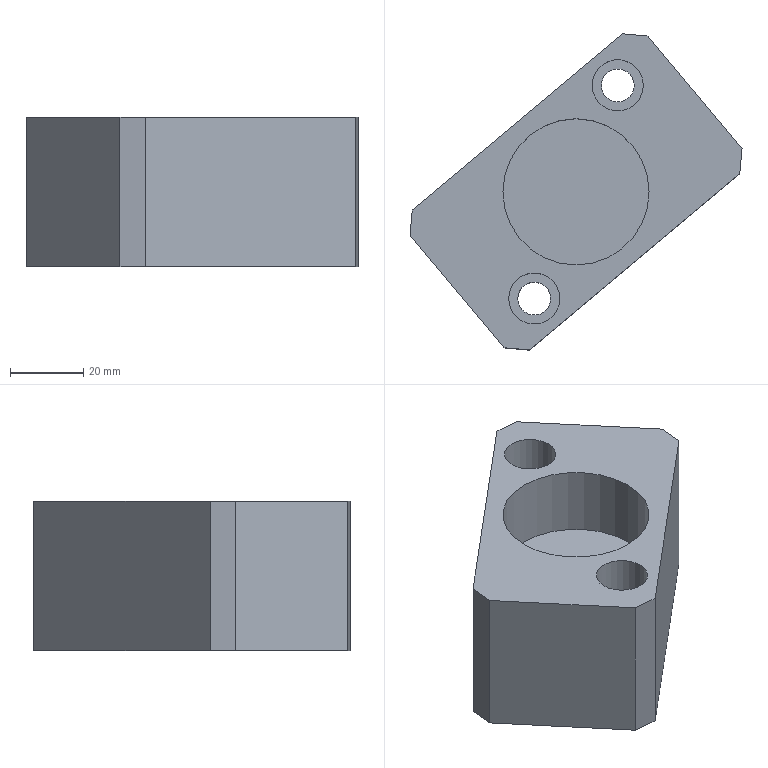Part | NX | features solid 2 | 1 solid | 18 faces | box 90.825 x 86.511 x 41 mm | volume 139314 mm3 | plane 13 | cylinder 5 | commonest cylinder face diameters 9 x2 14 x2 40 x1
STEP:
#1=CARTESIAN_POINT('',(-247.002,-330.511,-169.));
#2=VERTEX_POINT('',#1);
#3=CARTESIAN_POINT('',(-240.002,-330.511,-169.));
#4=DIRECTION('',(0.,0.,-1.));
#5=DIRECTION('',(-1.,0.,0.));
#6=AXIS2_PLACEMENT_3D('',#3,#4,#5);
#7=CIRCLE('',#6,7.);
#8=EDGE_CURVE('',#2,#2,#7,.T.);
#9=ORIENTED_EDGE('',*,*,#8,.T.);
#10=EDGE_LOOP('',(#9));
#11=FACE_BOUND('',#10,.T.);
#12=CARTESIAN_POINT('',(-269.851,-388.846,-169.));
#13=VERTEX_POINT('',#12);
#14=CARTESIAN_POINT('',(-262.851,-388.846,-169.));
#15=DIRECTION('',(0.,0.,-1.));
#16=DIRECTION('',(-1.,0.,0.));
#17=AXIS2_PLACEMENT_3D('',#14,#15,#16);
#18=CIRCLE('',#17,7.);
#19=EDGE_CURVE('',#13,#13,#18,.T.);
#20=ORIENTED_EDGE('',*,*,#19,.T.);
#21=EDGE_LOOP('',(#20));
#22=FACE_BOUND('',#21,.T.);
#23=CARTESIAN_POINT('',(-206.014,-347.681,-169.));
#24=VERTEX_POINT('',#23);
#25=CARTESIAN_POINT('',(-231.725,-317.039,-169.));
#26=VERTEX_POINT('',#25);
#27=CARTESIAN_POINT('',(-206.014,-347.681,-169.));
#28=DIRECTION('',(-0.6428,0.766,0.));
#29=VECTOR('',#28,1000.);
#30=LINE('',#27,#29);
#31=EDGE_CURVE('',#24,#26,#30,.T.);
#32=ORIENTED_EDGE('',*,*,#31,.T.);
#33=CARTESIAN_POINT('',(-238.77,-316.423,-169.));
#34=VERTEX_POINT('',#33);
#35=CARTESIAN_POINT('',(-259.902,-314.574,-169.));
#36=DIRECTION('',(0.9962,-0.08716,0.));
#37=VECTOR('',#36,1000.);
#38=LINE('',#35,#37);
#39=EDGE_CURVE('',#26,#34,#38,.F.);
#40=ORIENTED_EDGE('',*,*,#39,.T.);
#41=CARTESIAN_POINT('',(-296.223,-364.632,-169.));
#42=VERTEX_POINT('',#41);
#43=CARTESIAN_POINT('',(-296.223,-364.632,-169.));
#44=DIRECTION('',(-0.766,-0.6428,0.));
#45=VECTOR('',#44,1000.);
#46=LINE('',#43,#45);
#47=EDGE_CURVE('',#34,#42,#46,.T.);
#48=ORIENTED_EDGE('',*,*,#47,.T.);
#49=CARTESIAN_POINT('',(-296.839,-371.676,-169.));
#50=VERTEX_POINT('',#49);
#51=CARTESIAN_POINT('',(-298.996,-396.331,-169.));
#52=DIRECTION('',(0.08716,0.9962,0.));
#53=VECTOR('',#52,1000.);
#54=LINE('',#51,#53);
#55=EDGE_CURVE('',#42,#50,#54,.F.);
#56=ORIENTED_EDGE('',*,*,#55,.T.);
#57=CARTESIAN_POINT('',(-271.128,-402.318,-169.));
#58=VERTEX_POINT('',#57);
#59=CARTESIAN_POINT('',(-271.128,-402.318,-169.));
#60=DIRECTION('',(0.6428,-0.766,0.));
#61=VECTOR('',#60,1000.);
#62=LINE('',#59,#61);
#63=EDGE_CURVE('',#50,#58,#62,.T.);
#64=ORIENTED_EDGE('',*,*,#63,.T.);
#65=CARTESIAN_POINT('',(-264.084,-402.934,-169.));
#66=VERTEX_POINT('',#65);
#67=CARTESIAN_POINT('',(-267.606,-402.626,-169.));
#68=DIRECTION('',(-0.9962,0.08716,0.));
#69=VECTOR('',#68,1000.);
#70=LINE('',#67,#69);
#71=EDGE_CURVE('',#58,#66,#70,.F.);
#72=ORIENTED_EDGE('',*,*,#71,.T.);
#73=CARTESIAN_POINT('',(-206.63,-354.725,-169.));
#74=VERTEX_POINT('',#73);
#75=CARTESIAN_POINT('',(-264.084,-402.934,-169.));
#76=DIRECTION('',(0.766,0.6428,0.));
#77=VECTOR('',#76,1000.);
#78=LINE('',#75,#77);
#79=EDGE_CURVE('',#66,#74,#78,.T.);
#80=ORIENTED_EDGE('',*,*,#79,.T.);
#81=CARTESIAN_POINT('',(-210.944,-404.034,-169.));
#82=DIRECTION('',(-0.08716,-0.9962,0.));
#83=VECTOR('',#82,1000.);
#84=LINE('',#81,#83);
#85=EDGE_CURVE('',#74,#24,#84,.F.);
#86=ORIENTED_EDGE('',*,*,#85,.T.);
#87=EDGE_LOOP('',(#32,#40,#48,#56,#64,#72,#80,#86));
#88=FACE_BOUND('',#87,.T.);
#89=CARTESIAN_POINT('',(-271.427,-359.679,-169.));
#90=VERTEX_POINT('',#89);
#91=CARTESIAN_POINT('',(-251.427,-359.679,-169.));
#92=DIRECTION('',(0.,0.,1.));
#93=DIRECTION('',(-1.,0.,0.));
#94=AXIS2_PLACEMENT_3D('',#91,#92,#93);
#95=CIRCLE('',#94,20.);
#96=EDGE_CURVE('',#90,#90,#95,.F.);
#97=ORIENTED_EDGE('',*,*,#96,.T.);
#98=EDGE_LOOP('',(#97));
#99=FACE_BOUND('',#98,.T.);
#100=CARTESIAN_POINT('',(-267.297,-399.104,-169.));
#101=DIRECTION('',(0.,0.,1.));
#102=DIRECTION('',(-1.,0.,0.));
#103=AXIS2_PLACEMENT_3D('',#100,#101,#102);
#104=PLANE('',#103);
#105=ADVANCED_FACE('',(#11,#22,#88,#99),#104,.T.);
#106=ORIENTED_EDGE('',*,*,#63,.F.);
#107=CARTESIAN_POINT('',(-296.839,-371.676,-210.));
#108=VERTEX_POINT('',#107);
#109=CARTESIAN_POINT('',(-296.839,-371.676,-209.));
#110=DIRECTION('',(0.,0.,-1.));
#111=VECTOR('',#110,1000.);
#112=LINE('',#109,#111);
#113=EDGE_CURVE('',#50,#108,#112,.T.);
#114=ORIENTED_EDGE('',*,*,#113,.T.);
#115=CARTESIAN_POINT('',(-271.128,-402.318,-210.));
#116=VERTEX_POINT('',#115);
#117=CARTESIAN_POINT('',(-331.881,-329.915,-210.));
#118=DIRECTION('',(0.6428,-0.766,0.));
#119=VECTOR('',#118,1000.);
#120=LINE('',#117,#119);
#121=EDGE_CURVE('',#108,#116,#120,.T.);
#122=ORIENTED_EDGE('',*,*,#121,.T.);
#123=CARTESIAN_POINT('',(-271.128,-402.318,-209.));
#124=DIRECTION('',(0.,0.,1.));
#125=VECTOR('',#124,1000.);
#126=LINE('',#123,#125);
#127=EDGE_CURVE('',#116,#58,#126,.T.);
#128=ORIENTED_EDGE('',*,*,#127,.T.);
#129=EDGE_LOOP('',(#106,#114,#122,#128));
#130=FACE_BOUND('',#129,.T.);
#131=CARTESIAN_POINT('',(-296.839,-371.676,-209.));
#132=DIRECTION('',(-0.766,-0.6428,0.));
#133=DIRECTION('',(0.6428,-0.766,0.));
#134=AXIS2_PLACEMENT_3D('',#131,#132,#133);
#135=PLANE('',#134);
#136=ADVANCED_FACE('',(#130),#135,.T.);
#137=CARTESIAN_POINT('',(-264.084,-402.934,-210.));
#138=VERTEX_POINT('',#137);
#139=CARTESIAN_POINT('',(-206.63,-354.725,-210.));
#140=VERTEX_POINT('',#139);
#141=CARTESIAN_POINT('',(-362.898,-485.85,-210.));
#142=DIRECTION('',(0.766,0.6428,0.));
#143=VECTOR('',#142,1000.);
#144=LINE('',#141,#143);
#145=EDGE_CURVE('',#138,#140,#144,.T.);
#146=ORIENTED_EDGE('',*,*,#145,.T.);
#147=CARTESIAN_POINT('',(-206.63,-354.725,-209.));
#148=DIRECTION('',(0.,0.,1.));
#149=VECTOR('',#148,1000.);
#150=LINE('',#147,#149);
#151=EDGE_CURVE('',#140,#74,#150,.T.);
#152=ORIENTED_EDGE('',*,*,#151,.T.);
#153=ORIENTED_EDGE('',*,*,#79,.F.);
#154=CARTESIAN_POINT('',(-264.084,-402.934,-209.));
#155=DIRECTION('',(0.,0.,-1.));
#156=VECTOR('',#155,1000.);
#157=LINE('',#154,#156);
#158=EDGE_CURVE('',#66,#138,#157,.T.);
#159=ORIENTED_EDGE('',*,*,#158,.T.);
#160=EDGE_LOOP('',(#146,#152,#153,#159));
#161=FACE_BOUND('',#160,.T.);
#162=CARTESIAN_POINT('',(-264.084,-402.934,-209.));
#163=DIRECTION('',(0.6428,-0.766,0.));
#164=DIRECTION('',(0.766,0.6428,0.));
#165=AXIS2_PLACEMENT_3D('',#162,#163,#164);
#166=PLANE('',#165);
#167=ADVANCED_FACE('',(#161),#166,.T.);
#168=CARTESIAN_POINT('',(-206.014,-347.681,-210.));
#169=VERTEX_POINT('',#168);
#170=CARTESIAN_POINT('',(-231.725,-317.039,-210.));
#171=VERTEX_POINT('',#170);
#172=CARTESIAN_POINT('',(-266.767,-275.278,-210.));
#173=DIRECTION('',(-0.6428,0.766,0.));
#174=VECTOR('',#173,1000.);
#175=LINE('',#172,#174);
#176=EDGE_CURVE('',#169,#171,#175,.T.);
#177=ORIENTED_EDGE('',*,*,#176,.T.);
#178=CARTESIAN_POINT('',(-231.725,-317.039,-209.));
#179=DIRECTION('',(0.,0.,1.));
#180=VECTOR('',#179,1000.);
#181=LINE('',#178,#180);
#182=EDGE_CURVE('',#171,#26,#181,.T.);
#183=ORIENTED_EDGE('',*,*,#182,.T.);
#184=ORIENTED_EDGE('',*,*,#31,.F.);
#185=CARTESIAN_POINT('',(-206.014,-347.681,-209.));
#186=DIRECTION('',(0.,0.,-1.));
#187=VECTOR('',#186,1000.);
#188=LINE('',#185,#187);
#189=EDGE_CURVE('',#24,#169,#188,.T.);
#190=ORIENTED_EDGE('',*,*,#189,.T.);
#191=EDGE_LOOP('',(#177,#183,#184,#190));
#192=FACE_BOUND('',#191,.T.);
#193=CARTESIAN_POINT('',(-206.014,-347.681,-209.));
#194=DIRECTION('',(0.766,0.6428,0.));
#195=DIRECTION('',(-0.6428,0.766,0.));
#196=AXIS2_PLACEMENT_3D('',#193,#194,#195);
#197=PLANE('',#196);
#198=ADVANCED_FACE('',(#192),#197,.T.);
#199=ORIENTED_EDGE('',*,*,#47,.F.);
#200=CARTESIAN_POINT('',(-238.77,-316.423,-210.));
#201=VERTEX_POINT('',#200);
#202=CARTESIAN_POINT('',(-238.77,-316.423,-209.));
#203=DIRECTION('',(0.,0.,-1.));
#204=VECTOR('',#203,1000.);
#205=LINE('',#202,#204);
#206=EDGE_CURVE('',#34,#201,#205,.T.);
#207=ORIENTED_EDGE('',*,*,#206,.T.);
#208=CARTESIAN_POINT('',(-296.223,-364.632,-210.));
#209=VERTEX_POINT('',#208);
#210=CARTESIAN_POINT('',(-395.038,-447.548,-210.));
#211=DIRECTION('',(-0.766,-0.6428,0.));
#212=VECTOR('',#211,1000.);
#213=LINE('',#210,#212);
#214=EDGE_CURVE('',#201,#209,#213,.T.);
#215=ORIENTED_EDGE('',*,*,#214,.T.);
#216=CARTESIAN_POINT('',(-296.223,-364.632,-209.));
#217=DIRECTION('',(0.,0.,1.));
#218=VECTOR('',#217,1000.);
#219=LINE('',#216,#218);
#220=EDGE_CURVE('',#209,#42,#219,.T.);
#221=ORIENTED_EDGE('',*,*,#220,.T.);
#222=EDGE_LOOP('',(#199,#207,#215,#221));
#223=FACE_BOUND('',#222,.T.);
#224=CARTESIAN_POINT('',(-238.77,-316.423,-209.));
#225=DIRECTION('',(-0.6428,0.766,0.));
#226=DIRECTION('',(-0.766,-0.6428,0.));
#227=AXIS2_PLACEMENT_3D('',#224,#225,#226);
#228=PLANE('',#227);
#229=ADVANCED_FACE('',(#223),#228,.T.);
#230=CARTESIAN_POINT('',(-244.502,-330.511,-210.));
#231=VERTEX_POINT('',#230);
#232=CARTESIAN_POINT('',(-240.002,-330.511,-210.));
#233=DIRECTION('',(0.,0.,-1.));
#234=DIRECTION('',(-1.,0.,0.));
#235=AXIS2_PLACEMENT_3D('',#232,#233,#234);
#236=CIRCLE('',#235,4.5);
#237=EDGE_CURVE('',#231,#231,#236,.T.);
#238=ORIENTED_EDGE('',*,*,#237,.F.);
#239=EDGE_LOOP('',(#238));
#240=FACE_BOUND('',#239,.T.);
#241=CARTESIAN_POINT('',(-267.351,-388.846,-210.));
#242=VERTEX_POINT('',#241);
#243=CARTESIAN_POINT('',(-262.851,-388.846,-210.));
#244=DIRECTION('',(0.,0.,-1.));
#245=DIRECTION('',(-1.,0.,0.));
#246=AXIS2_PLACEMENT_3D('',#243,#244,#245);
#247=CIRCLE('',#246,4.5);
#248=EDGE_CURVE('',#242,#242,#247,.T.);
#249=ORIENTED_EDGE('',*,*,#248,.F.);
#250=EDGE_LOOP('',(#249));
#251=FACE_BOUND('',#250,.T.);
#252=ORIENTED_EDGE('',*,*,#214,.F.);
#253=CARTESIAN_POINT('',(-231.725,-317.039,-210.));
#254=DIRECTION('',(-0.9962,0.08716,0.));
#255=VECTOR('',#254,1000.);
#256=LINE('',#253,#255);
#257=EDGE_CURVE('',#201,#171,#256,.F.);
#258=ORIENTED_EDGE('',*,*,#257,.T.);
#259=ORIENTED_EDGE('',*,*,#176,.F.);
#260=CARTESIAN_POINT('',(-206.63,-354.725,-210.));
#261=DIRECTION('',(0.08716,0.9962,0.));
#262=VECTOR('',#261,1000.);
#263=LINE('',#260,#262);
#264=EDGE_CURVE('',#169,#140,#263,.F.);
#265=ORIENTED_EDGE('',*,*,#264,.T.);
#266=ORIENTED_EDGE('',*,*,#145,.F.);
#267=CARTESIAN_POINT('',(-271.128,-402.318,-210.));
#268=DIRECTION('',(0.9962,-0.08716,0.));
#269=VECTOR('',#268,1000.);
#270=LINE('',#267,#269);
#271=EDGE_CURVE('',#138,#116,#270,.F.);
#272=ORIENTED_EDGE('',*,*,#271,.T.);
#273=ORIENTED_EDGE('',*,*,#121,.F.);
#274=CARTESIAN_POINT('',(-296.223,-364.632,-210.));
#275=DIRECTION('',(-0.08716,-0.9962,0.));
#276=VECTOR('',#275,1000.);
#277=LINE('',#274,#276);
#278=EDGE_CURVE('',#108,#209,#277,.F.);
#279=ORIENTED_EDGE('',*,*,#278,.T.);
#280=EDGE_LOOP('',(#252,#258,#259,#265,#266,#272,#273,#279));
#281=FACE_BOUND('',#280,.T.);
#282=CARTESIAN_POINT('',(-426.866,-409.617,-210.));
#283=DIRECTION('',(0.,0.,1.));
#284=DIRECTION('',(-1.,0.,0.));
#285=AXIS2_PLACEMENT_3D('',#282,#283,#284);
#286=PLANE('',#285);
#287=ADVANCED_FACE('',(#240,#251,#281),#286,.F.);
#288=ORIENTED_EDGE('',*,*,#271,.F.);
#289=ORIENTED_EDGE('',*,*,#158,.F.);
#290=ORIENTED_EDGE('',*,*,#71,.F.);
#291=ORIENTED_EDGE('',*,*,#127,.F.);
#292=EDGE_LOOP('',(#288,#289,#290,#291));
#293=FACE_BOUND('',#292,.T.);
#294=CARTESIAN_POINT('',(-271.128,-402.318,-209.));
#295=DIRECTION('',(0.08716,0.9962,0.));
#296=DIRECTION('',(-0.9962,0.08716,0.));
#297=AXIS2_PLACEMENT_3D('',#294,#295,#296);
#298=PLANE('',#297);
#299=ADVANCED_FACE('',(#293),#298,.F.);
#300=ORIENTED_EDGE('',*,*,#278,.F.);
#301=ORIENTED_EDGE('',*,*,#113,.F.);
#302=ORIENTED_EDGE('',*,*,#55,.F.);
#303=ORIENTED_EDGE('',*,*,#220,.F.);
#304=EDGE_LOOP('',(#300,#301,#302,#303));
#305=FACE_BOUND('',#304,.T.);
#306=CARTESIAN_POINT('',(-296.223,-364.632,-209.));
#307=DIRECTION('',(0.9962,-0.08716,0.));
#308=DIRECTION('',(0.08716,0.9962,0.));
#309=AXIS2_PLACEMENT_3D('',#306,#307,#308);
#310=PLANE('',#309);
#311=ADVANCED_FACE('',(#305),#310,.F.);
#312=ORIENTED_EDGE('',*,*,#264,.F.);
#313=ORIENTED_EDGE('',*,*,#189,.F.);
#314=ORIENTED_EDGE('',*,*,#85,.F.);
#315=ORIENTED_EDGE('',*,*,#151,.F.);
#316=EDGE_LOOP('',(#312,#313,#314,#315));
#317=FACE_BOUND('',#316,.T.);
#318=CARTESIAN_POINT('',(-206.63,-354.725,-209.));
#319=DIRECTION('',(-0.9962,0.08716,0.));
#320=DIRECTION('',(-0.08716,-0.9962,0.));
#321=AXIS2_PLACEMENT_3D('',#318,#319,#320);
#322=PLANE('',#321);
#323=ADVANCED_FACE('',(#317),#322,.F.);
#324=ORIENTED_EDGE('',*,*,#257,.F.);
#325=ORIENTED_EDGE('',*,*,#206,.F.);
#326=ORIENTED_EDGE('',*,*,#39,.F.);
#327=ORIENTED_EDGE('',*,*,#182,.F.);
#328=EDGE_LOOP('',(#324,#325,#326,#327));
#329=FACE_BOUND('',#328,.T.);
#330=CARTESIAN_POINT('',(-231.725,-317.039,-209.));
#331=DIRECTION('',(-0.08716,-0.9962,0.));
#332=DIRECTION('',(0.9962,-0.08716,0.));
#333=AXIS2_PLACEMENT_3D('',#330,#331,#332);
#334=PLANE('',#333);
#335=ADVANCED_FACE('',(#329),#334,.F.);
#336=ORIENTED_EDGE('',*,*,#96,.F.);
#337=EDGE_LOOP('',(#336));
#338=FACE_BOUND('',#337,.T.);
#339=CARTESIAN_POINT('',(-271.427,-359.679,-188.));
#340=VERTEX_POINT('',#339);
#341=CARTESIAN_POINT('',(-251.427,-359.679,-188.));
#342=DIRECTION('',(0.,0.,1.));
#343=DIRECTION('',(-1.,0.,0.));
#344=AXIS2_PLACEMENT_3D('',#341,#342,#343);
#345=CIRCLE('',#344,20.);
#346=EDGE_CURVE('',#340,#340,#345,.T.);
#347=ORIENTED_EDGE('',*,*,#346,.F.);
#348=EDGE_LOOP('',(#347));
#349=FACE_BOUND('',#348,.T.);
#350=CARTESIAN_POINT('',(-251.427,-359.679,-78.));
#351=DIRECTION('',(0.,0.,-1.));
#352=DIRECTION('',(1.,0.,0.));
#353=AXIS2_PLACEMENT_3D('',#350,#351,#352);
#354=CYLINDRICAL_SURFACE('',#353,20.);
#355=ADVANCED_FACE('',(#338,#349),#354,.F.);
#356=ORIENTED_EDGE('',*,*,#346,.T.);
#357=EDGE_LOOP('',(#356));
#358=FACE_BOUND('',#357,.T.);
#359=CARTESIAN_POINT('',(-251.427,-359.679,-188.));
#360=DIRECTION('',(0.,0.,1.));
#361=DIRECTION('',(-1.,0.,0.));
#362=AXIS2_PLACEMENT_3D('',#359,#360,#361);
#363=PLANE('',#362);
#364=ADVANCED_FACE('',(#358),#363,.T.);
#365=CARTESIAN_POINT('',(-258.351,-388.846,-190.));
#366=VERTEX_POINT('',#365);
#367=CARTESIAN_POINT('',(-262.851,-388.846,-190.));
#368=DIRECTION('',(0.,0.,1.));
#369=DIRECTION('',(1.,0.,0.));
#370=AXIS2_PLACEMENT_3D('',#367,#368,#369);
#371=CIRCLE('',#370,4.5);
#372=EDGE_CURVE('',#366,#366,#371,.F.);
#373=ORIENTED_EDGE('',*,*,#372,.F.);
#374=EDGE_LOOP('',(#373));
#375=FACE_BOUND('',#374,.T.);
#376=ORIENTED_EDGE('',*,*,#248,.T.);
#377=EDGE_LOOP('',(#376));
#378=FACE_BOUND('',#377,.T.);
#379=CARTESIAN_POINT('',(-262.851,-388.846,-230.));
#380=DIRECTION('',(0.,0.,1.));
#381=DIRECTION('',(-1.,0.,0.));
#382=AXIS2_PLACEMENT_3D('',#379,#380,#381);
#383=CYLINDRICAL_SURFACE('',#382,4.5);
#384=ADVANCED_FACE('',(#375,#378),#383,.F.);
#385=ORIENTED_EDGE('',*,*,#372,.T.);
#386=EDGE_LOOP('',(#385));
#387=FACE_BOUND('',#386,.T.);
#388=CARTESIAN_POINT('',(-269.851,-388.846,-190.));
#389=VERTEX_POINT('',#388);
#390=CARTESIAN_POINT('',(-262.851,-388.846,-190.));
#391=DIRECTION('',(0.,0.,-1.));
#392=DIRECTION('',(-1.,0.,0.));
#393=AXIS2_PLACEMENT_3D('',#390,#391,#392);
#394=CIRCLE('',#393,7.);
#395=EDGE_CURVE('',#389,#389,#394,.T.);
#396=ORIENTED_EDGE('',*,*,#395,.F.);
#397=EDGE_LOOP('',(#396));
#398=FACE_BOUND('',#397,.T.);
#399=CARTESIAN_POINT('',(-262.851,-388.846,-190.));
#400=DIRECTION('',(0.,0.,-1.));
#401=DIRECTION('',(1.,0.,0.));
#402=AXIS2_PLACEMENT_3D('',#399,#400,#401);
#403=PLANE('',#402);
#404=ADVANCED_FACE('',(#387,#398),#403,.F.);
#405=ORIENTED_EDGE('',*,*,#19,.F.);
#406=EDGE_LOOP('',(#405));
#407=FACE_BOUND('',#406,.T.);
#408=ORIENTED_EDGE('',*,*,#395,.T.);
#409=EDGE_LOOP('',(#408));
#410=FACE_BOUND('',#409,.T.);
#411=CARTESIAN_POINT('',(-262.851,-388.846,-190.));
#412=DIRECTION('',(0.,0.,1.));
#413=DIRECTION('',(-1.,0.,0.));
#414=AXIS2_PLACEMENT_3D('',#411,#412,#413);
#415=CYLINDRICAL_SURFACE('',#414,7.);
#416=ADVANCED_FACE('',(#407,#410),#415,.F.);
#417=CARTESIAN_POINT('',(-235.502,-330.511,-190.));
#418=VERTEX_POINT('',#417);
#419=CARTESIAN_POINT('',(-240.002,-330.511,-190.));
#420=DIRECTION('',(0.,0.,1.));
#421=DIRECTION('',(1.,0.,0.));
#422=AXIS2_PLACEMENT_3D('',#419,#420,#421);
#423=CIRCLE('',#422,4.5);
#424=EDGE_CURVE('',#418,#418,#423,.F.);
#425=ORIENTED_EDGE('',*,*,#424,.F.);
#426=EDGE_LOOP('',(#425));
#427=FACE_BOUND('',#426,.T.);
#428=ORIENTED_EDGE('',*,*,#237,.T.);
#429=EDGE_LOOP('',(#428));
#430=FACE_BOUND('',#429,.T.);
#431=CARTESIAN_POINT('',(-240.002,-330.511,-230.));
#432=DIRECTION('',(0.,0.,1.));
#433=DIRECTION('',(-1.,0.,0.));
#434=AXIS2_PLACEMENT_3D('',#431,#432,#433);
#435=CYLINDRICAL_SURFACE('',#434,4.5);
#436=ADVANCED_FACE('',(#427,#430),#435,.F.);
#437=ORIENTED_EDGE('',*,*,#424,.T.);
#438=EDGE_LOOP('',(#437));
#439=FACE_BOUND('',#438,.T.);
#440=CARTESIAN_POINT('',(-247.002,-330.511,-190.));
#441=VERTEX_POINT('',#440);
#442=CARTESIAN_POINT('',(-240.002,-330.511,-190.));
#443=DIRECTION('',(0.,0.,-1.));
#444=DIRECTION('',(-1.,0.,0.));
#445=AXIS2_PLACEMENT_3D('',#442,#443,#444);
#446=CIRCLE('',#445,7.);
#447=EDGE_CURVE('',#441,#441,#446,.T.);
#448=ORIENTED_EDGE('',*,*,#447,.F.);
#449=EDGE_LOOP('',(#448));
#450=FACE_BOUND('',#449,.T.);
#451=CARTESIAN_POINT('',(-240.002,-330.511,-190.));
#452=DIRECTION('',(0.,0.,-1.));
#453=DIRECTION('',(1.,0.,0.));
#454=AXIS2_PLACEMENT_3D('',#451,#452,#453);
#455=PLANE('',#454);
#456=ADVANCED_FACE('',(#439,#450),#455,.F.);
#457=ORIENTED_EDGE('',*,*,#8,.F.);
#458=EDGE_LOOP('',(#457));
#459=FACE_BOUND('',#458,.T.);
#460=ORIENTED_EDGE('',*,*,#447,.T.);
#461=EDGE_LOOP('',(#460));
#462=FACE_BOUND('',#461,.T.);
#463=CARTESIAN_POINT('',(-240.002,-330.511,-190.));
#464=DIRECTION('',(0.,0.,1.));
#465=DIRECTION('',(-1.,0.,0.));
#466=AXIS2_PLACEMENT_3D('',#463,#464,#465);
#467=CYLINDRICAL_SURFACE('',#466,7.);
#468=ADVANCED_FACE('',(#459,#462),#467,.F.);
#469=CLOSED_SHELL('',(#105,#136,#167,#198,#229,#287,#299,#311,#323,#335,#355,#364,#384,#404,#416,#436,#456,#468));
#470=MANIFOLD_SOLID_BREP('',#469);
#471=(LENGTH_UNIT()NAMED_UNIT(*)SI_UNIT(.MILLI.,.METRE.));
#472=UNCERTAINTY_MEASURE_WITH_UNIT(LENGTH_MEASURE(0.00001),#471,'','');
#473=(NAMED_UNIT(*)PLANE_ANGLE_UNIT()SI_UNIT($,.RADIAN.));
#474=(NAMED_UNIT(*)SI_UNIT($,.STERADIAN.)SOLID_ANGLE_UNIT());
#475=(GEOMETRIC_REPRESENTATION_CONTEXT(3)GLOBAL_UNCERTAINTY_ASSIGNED_CONTEXT((#472))GLOBAL_UNIT_ASSIGNED_CONTEXT((#471,#473,#474))REPRESENTATION_CONTEXT('',''));
#476=ADVANCED_BREP_SHAPE_REPRESENTATION('',(#470),#475);